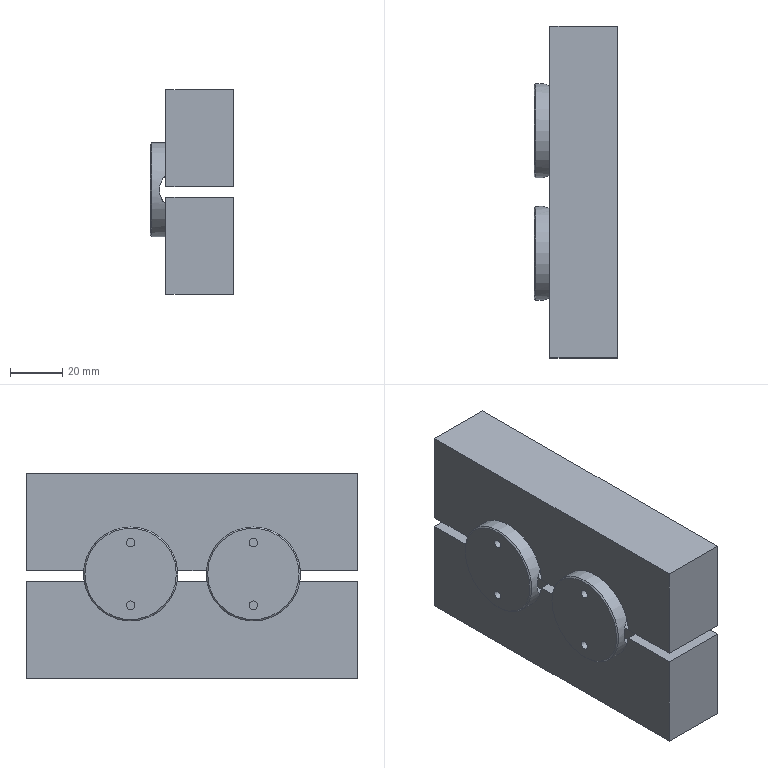CAM job | NX | 3+2 milling, drilling | part box 32 x 127 x 78.432 mm
Tools:
number,name,description,diameter,corner_radius,flute_length,length,flutes
6,D6,平底铣刀-粗,6.0,0.0,25.0,75.0,2
9,D10,平底铣刀-粗,10.0,0.0,35.0,75.0,2
10,D10-J,平底铣刀-精,10.0,0.0,35.0,75.0,2
1,D80R0.8飞刀,圆鼻刀-粗,80.0,0.8,50.0,75.0,2
1,D80R0.8飞刀-J,圆鼻刀-精,80.0,0.8,50.0,75.0,2
2,D6倒角刀,倒角刀,6.0,0.0,3.0,25.0,2
17,R3,圆球刀,6.0,3.0,12.0,50.0,2
21,M4X0.7,丝锥,3.3,0.0,35.0,50.0,2
13,钻头3.3,Twist Drill 3.3 mm,3.3,0.0,35.0,35.008,2
Operations:
program,operation,operation_type,tool,method,geometry_group,spindle_rpm,surface_speed,feed_per_tooth,feed_cut,feed_plunge,cut_length_mm,path_length_mm,cut_time_min,machine_time_min
C,底壁铣分层开粗-中_COPY,VolumeBased25DMillingOperation,D10,分层开粗-切深K-步距G,W-C,8000.0,251.327,0.125,2000.0,100.0,2420.943,2735.254,1.21,1.242
C,底壁铣精光底面-中_COPY,VolumeBased25DMillingOperation,D10-J,精光步距切深关,W-C,8000.0,251.32,0.0625,1000.0,100.0,339.06,437.943,0.3391,0.3489
C,C0.3封闭铣廓倒角6X45L_COPY,PlanarMilling,D6倒角刀,爬面_倒角-切深0-步距G,W-C,7000.0,131.0,0.1071,1500.0,100.0,243.848,482.852,0.1626,0.1865
C,底壁铣精光侧面-中-选底面_COPY,VolumeBased25DMillingOperation,D10-J,侧刃精光-切深K-步距G,W-C,8000.0,251.32,0.0625,1000.0,100.0,182.474,302.354,0.1825,0.1945
B,底壁铣飞面一刀开粗_COPY,VolumeBased25DMillingOperation,D80R0.8飞刀,分层开粗-切深K-步距G,W-B,2800.0,703.696,0.5357,3000.0,100.0,764.625,1360.47,0.2549,0.3145
B,底壁铣飞面一刀精光_COPY,VolumeBased25DMillingOperation,D80R0.8飞刀-J,侧刃精光-切深K-步距G,W-B,4000.0,1005.28,0.125,1000.0,100.0,190.96,226.96,0.191,0.1946
B,钻倒角_2,Operation,D6倒角刀,METHOD,W-B,8000.0,150.796,0.0625,1000.0,0.0,20.8,191.832,0.0208,0.0379
B,底壁铣倒角_COPY_1,VolumeBased25DMillingOperation,D6倒角刀,爬面_倒角-切深0-步距G,W-B,6500.0,122.519,0.1154,1500.0,100.0,249.186,372.163,0.1661,0.1784
A,顶面,FaceMilling,D80R0.8飞刀,侧刃精光-切深K-步距G,W-A,4000.0,1005.31,0.125,1000.0,100.0,177.0,213.0,0.177,0.1806
A,型腔铣开粗-中_COPY,CavityMilling,D6,分层开粗-切深K-步距G,W-A,8000.0,251.32,0.25,4000.0,100.0,19602.132,20170.947,4.901,4.982
A,打点-深0.8,Operation,D6倒角刀,NONE,W-A,8000.0,150.796,0.0312,500.0,90.0,7.2,158.224,0.0144,0.0295
A,通孔-M4螺纹底孔,Operation,钻头3.3,NONE,W-A,3000.0,31.102,0.05,300.0,90.0,67.966,279.756,0.2266,0.2477
A,仅选体,SurfaceContour,D6倒角刀,METHOD,W-A,8000.0,150.796,0.1875,3000.0,100.0,164.472,374.307,0.0548,0.0758
A,钻倒角_1,Operation,D6倒角刀,METHOD,W-A,8000.0,150.796,0.0312,500.0,0.0,20.8,191.832,0.0416,0.0587
A,底壁铣倒角_COPY,VolumeBased25DMillingOperation,D6倒角刀,爬面_倒角-切深0-步距G,W-A,6500.0,122.519,0.1154,1500.0,100.0,206.89,395.146,0.1379,0.1568
A,曲面D6R3,SurfaceContour,R3,METHOD,W-A,6000.0,75.0,0.2083,3500.0,100.0,10088.612,10238.228,2.882,2.897
A,通孔-攻牙M4,Operation,M4X0.7,METHOD,W-A,600.0,6.22,0.0006,0.7,90.0,56.0,255.824,80.0,80.02
A,外形半精_2,VolumeBased25DMillingOperation,D10-J,METHOD,W-A,8000.0,251.327,0.0625,1000.0,100.0,299.026,491.14,0.299,0.3182